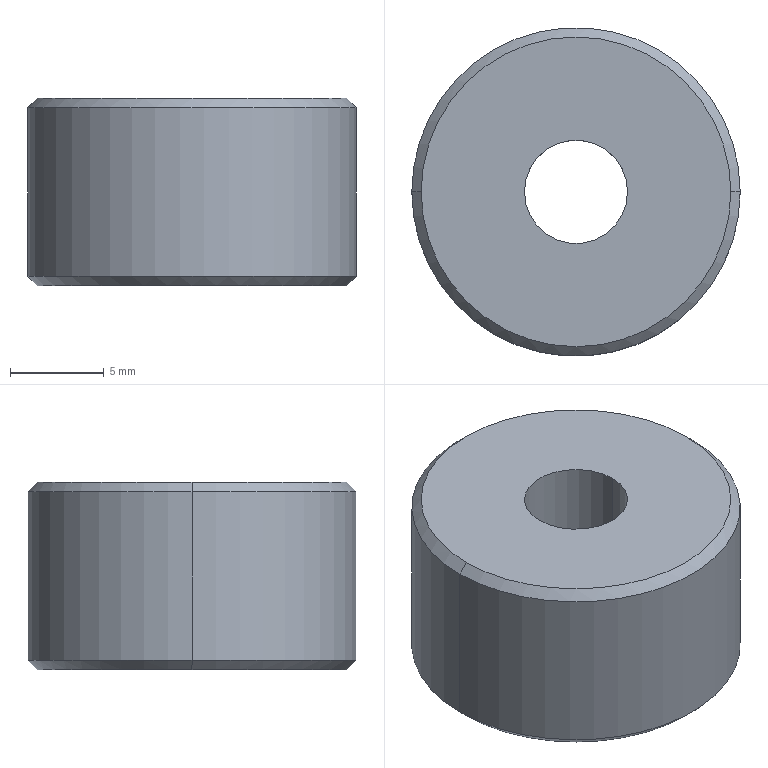Part | SolidWorks | features Chamfer 1, Extrusion 1, ICE 1 | 1 solid | 13 faces | box 17.5 x 17.5 x 10 mm | volume 1853 mm3 | cylinder 6 | cone 4 | plane 3 | commonest cylinder face diameters 5.5 x2 10 x2 17.5 x2
STEP:
#1=CARTESIAN_POINT('',(8.25,0.,10.));
#2=VERTEX_POINT('',#1);
#3=CARTESIAN_POINT('',(-8.25,0.,10.));
#4=VERTEX_POINT('',#3);
#5=CARTESIAN_POINT('',(0.,0.,10.));
#6=DIRECTION('',(0.,0.,1.));
#7=DIRECTION('',(1.,0.,0.));
#8=AXIS2_PLACEMENT_3D('',#5,#6,#7);
#9=CIRCLE('',#8,8.25);
#10=EDGE_CURVE('',#2,#4,#9,.T.);
#11=ORIENTED_EDGE('',*,*,#10,.F.);
#12=CARTESIAN_POINT('',(8.75,0.,9.5));
#13=VERTEX_POINT('',#12);
#14=CARTESIAN_POINT('',(8.25,0.,10.));
#15=DIRECTION('',(0.7071,0.,-0.7071));
#16=VECTOR('',#15,1000.);
#17=LINE('',#14,#16);
#18=EDGE_CURVE('',#2,#13,#17,.T.);
#19=ORIENTED_EDGE('',*,*,#18,.T.);
#20=CARTESIAN_POINT('',(-8.75,0.,9.5));
#21=VERTEX_POINT('',#20);
#22=CARTESIAN_POINT('',(0.,0.,9.5));
#23=DIRECTION('',(0.,0.,-1.));
#24=DIRECTION('',(1.,0.,0.));
#25=AXIS2_PLACEMENT_3D('',#22,#23,#24);
#26=CIRCLE('',#25,8.75);
#27=EDGE_CURVE('',#21,#13,#26,.T.);
#28=ORIENTED_EDGE('',*,*,#27,.F.);
#29=CARTESIAN_POINT('',(-8.25,0.,10.));
#30=DIRECTION('',(-0.7071,0.,-0.7071));
#31=VECTOR('',#30,1000.);
#32=LINE('',#29,#31);
#33=EDGE_CURVE('',#4,#21,#32,.T.);
#34=ORIENTED_EDGE('',*,*,#33,.F.);
#35=EDGE_LOOP('',(#11,#19,#28,#34));
#36=FACE_OUTER_BOUND('',#35,.T.);
#37=CARTESIAN_POINT('',(0.,0.,10.));
#38=DIRECTION('',(0.,0.,-1.));
#39=DIRECTION('',(-1.,0.,0.));
#40=AXIS2_PLACEMENT_3D('',#37,#38,#39);
#41=CONICAL_SURFACE('',#40,8.25,0.7854);
#42=ADVANCED_FACE('',(#36),#41,.T.);
#43=CARTESIAN_POINT('',(-8.25,0.,0.));
#44=VERTEX_POINT('',#43);
#45=CARTESIAN_POINT('',(8.25,0.,0.));
#46=VERTEX_POINT('',#45);
#47=CARTESIAN_POINT('',(0.,0.,0.));
#48=DIRECTION('',(0.,0.,-1.));
#49=DIRECTION('',(1.,0.,0.));
#50=AXIS2_PLACEMENT_3D('',#47,#48,#49);
#51=CIRCLE('',#50,8.25);
#52=EDGE_CURVE('',#44,#46,#51,.T.);
#53=ORIENTED_EDGE('',*,*,#52,.F.);
#54=CARTESIAN_POINT('',(-8.75,0.,0.5));
#55=VERTEX_POINT('',#54);
#56=CARTESIAN_POINT('',(-8.75,0.,0.5));
#57=DIRECTION('',(-0.7071,0.,0.7071));
#58=VECTOR('',#57,1000.);
#59=LINE('',#56,#58);
#60=EDGE_CURVE('',#44,#55,#59,.T.);
#61=ORIENTED_EDGE('',*,*,#60,.T.);
#62=CARTESIAN_POINT('',(8.75,0.,0.5));
#63=VERTEX_POINT('',#62);
#64=CARTESIAN_POINT('',(0.,0.,0.5));
#65=DIRECTION('',(0.,0.,1.));
#66=DIRECTION('',(1.,0.,0.));
#67=AXIS2_PLACEMENT_3D('',#64,#65,#66);
#68=CIRCLE('',#67,8.75);
#69=EDGE_CURVE('',#63,#55,#68,.T.);
#70=ORIENTED_EDGE('',*,*,#69,.F.);
#71=CARTESIAN_POINT('',(8.75,0.,0.5));
#72=DIRECTION('',(0.7071,0.,0.7071));
#73=VECTOR('',#72,1000.);
#74=LINE('',#71,#73);
#75=EDGE_CURVE('',#46,#63,#74,.T.);
#76=ORIENTED_EDGE('',*,*,#75,.F.);
#77=EDGE_LOOP('',(#53,#61,#70,#76));
#78=FACE_OUTER_BOUND('',#77,.T.);
#79=CARTESIAN_POINT('',(0.,0.,0.5));
#80=DIRECTION('',(0.,0.,1.));
#81=DIRECTION('',(1.,0.,0.));
#82=AXIS2_PLACEMENT_3D('',#79,#80,#81);
#83=CONICAL_SURFACE('',#82,8.75,0.7854);
#84=ADVANCED_FACE('',(#78),#83,.T.);
#85=CARTESIAN_POINT('',(5.,0.,5.5));
#86=VERTEX_POINT('',#85);
#87=CARTESIAN_POINT('',(-5.,0.,5.5));
#88=VERTEX_POINT('',#87);
#89=CARTESIAN_POINT('',(0.,0.,5.5));
#90=DIRECTION('',(0.,0.,-1.));
#91=DIRECTION('',(-1.,0.,0.));
#92=AXIS2_PLACEMENT_3D('',#89,#90,#91);
#93=CIRCLE('',#92,5.);
#94=EDGE_CURVE('',#86,#88,#93,.T.);
#95=ORIENTED_EDGE('',*,*,#94,.F.);
#96=CARTESIAN_POINT('',(5.,0.,0.));
#97=VERTEX_POINT('',#96);
#98=CARTESIAN_POINT('',(5.,0.,5.5));
#99=DIRECTION('',(0.,0.,-1.));
#100=VECTOR('',#99,1000.);
#101=LINE('',#98,#100);
#102=EDGE_CURVE('',#86,#97,#101,.T.);
#103=ORIENTED_EDGE('',*,*,#102,.T.);
#104=CARTESIAN_POINT('',(-5.,0.,0.));
#105=VERTEX_POINT('',#104);
#106=CARTESIAN_POINT('',(0.,0.,0.));
#107=DIRECTION('',(0.,0.,-1.));
#108=DIRECTION('',(-1.,0.,0.));
#109=AXIS2_PLACEMENT_3D('',#106,#107,#108);
#110=CIRCLE('',#109,5.);
#111=EDGE_CURVE('',#97,#105,#110,.T.);
#112=ORIENTED_EDGE('',*,*,#111,.T.);
#113=CARTESIAN_POINT('',(-5.,0.,5.5));
#114=DIRECTION('',(0.,0.,-1.));
#115=VECTOR('',#114,1000.);
#116=LINE('',#113,#115);
#117=EDGE_CURVE('',#88,#105,#116,.T.);
#118=ORIENTED_EDGE('',*,*,#117,.F.);
#119=EDGE_LOOP('',(#95,#103,#112,#118));
#120=FACE_OUTER_BOUND('',#119,.T.);
#121=CARTESIAN_POINT('',(0.,0.,5.5));
#122=DIRECTION('',(0.,0.,-1.));
#123=DIRECTION('',(-1.,0.,0.));
#124=AXIS2_PLACEMENT_3D('',#121,#122,#123);
#125=CYLINDRICAL_SURFACE('',#124,5.);
#126=ADVANCED_FACE('',(#120),#125,.F.);
#127=ORIENTED_EDGE('',*,*,#27,.T.);
#128=CARTESIAN_POINT('',(8.75,0.,10.));
#129=DIRECTION('',(0.,0.,-1.));
#130=VECTOR('',#129,1000.);
#131=LINE('',#128,#130);
#132=EDGE_CURVE('',#13,#63,#131,.T.);
#133=ORIENTED_EDGE('',*,*,#132,.T.);
#134=ORIENTED_EDGE('',*,*,#69,.T.);
#135=CARTESIAN_POINT('',(-8.75,0.,10.));
#136=DIRECTION('',(0.,0.,-1.));
#137=VECTOR('',#136,1000.);
#138=LINE('',#135,#137);
#139=EDGE_CURVE('',#21,#55,#138,.T.);
#140=ORIENTED_EDGE('',*,*,#139,.F.);
#141=EDGE_LOOP('',(#127,#133,#134,#140));
#142=FACE_OUTER_BOUND('',#141,.T.);
#143=CARTESIAN_POINT('',(0.,0.,10.));
#144=DIRECTION('',(0.,0.,-1.));
#145=DIRECTION('',(-1.,0.,0.));
#146=AXIS2_PLACEMENT_3D('',#143,#144,#145);
#147=CYLINDRICAL_SURFACE('',#146,8.75);
#148=ADVANCED_FACE('',(#142),#147,.T.);
#149=CARTESIAN_POINT('',(-2.75,0.,10.));
#150=VERTEX_POINT('',#149);
#151=CARTESIAN_POINT('',(2.75,0.,10.));
#152=VERTEX_POINT('',#151);
#153=CARTESIAN_POINT('',(0.,0.,10.));
#154=DIRECTION('',(0.,0.,1.));
#155=DIRECTION('',(1.,0.,0.));
#156=AXIS2_PLACEMENT_3D('',#153,#154,#155);
#157=CIRCLE('',#156,2.75);
#158=EDGE_CURVE('',#150,#152,#157,.T.);
#159=ORIENTED_EDGE('',*,*,#158,.T.);
#160=CARTESIAN_POINT('',(2.75,0.,5.5));
#161=VERTEX_POINT('',#160);
#162=CARTESIAN_POINT('',(2.75,0.,10.));
#163=DIRECTION('',(0.,0.,-1.));
#164=VECTOR('',#163,1000.);
#165=LINE('',#162,#164);
#166=EDGE_CURVE('',#152,#161,#165,.T.);
#167=ORIENTED_EDGE('',*,*,#166,.T.);
#168=CARTESIAN_POINT('',(-2.75,0.,5.5));
#169=VERTEX_POINT('',#168);
#170=CARTESIAN_POINT('',(0.,0.,5.5));
#171=DIRECTION('',(0.,0.,-1.));
#172=DIRECTION('',(-1.,0.,0.));
#173=AXIS2_PLACEMENT_3D('',#170,#171,#172);
#174=CIRCLE('',#173,2.75);
#175=EDGE_CURVE('',#161,#169,#174,.T.);
#176=ORIENTED_EDGE('',*,*,#175,.T.);
#177=CARTESIAN_POINT('',(-2.75,0.,10.));
#178=DIRECTION('',(0.,0.,-1.));
#179=VECTOR('',#178,1000.);
#180=LINE('',#177,#179);
#181=EDGE_CURVE('',#150,#169,#180,.T.);
#182=ORIENTED_EDGE('',*,*,#181,.F.);
#183=EDGE_LOOP('',(#159,#167,#176,#182));
#184=FACE_OUTER_BOUND('',#183,.T.);
#185=CARTESIAN_POINT('',(0.,0.,10.));
#186=DIRECTION('',(0.,0.,-1.));
#187=DIRECTION('',(-1.,0.,0.));
#188=AXIS2_PLACEMENT_3D('',#185,#186,#187);
#189=CYLINDRICAL_SURFACE('',#188,2.75);
#190=ADVANCED_FACE('',(#184),#189,.F.);
#191=ORIENTED_EDGE('',*,*,#166,.F.);
#192=CARTESIAN_POINT('',(0.,0.,10.));
#193=DIRECTION('',(0.,0.,1.));
#194=DIRECTION('',(1.,0.,0.));
#195=AXIS2_PLACEMENT_3D('',#192,#193,#194);
#196=CIRCLE('',#195,2.75);
#197=EDGE_CURVE('',#152,#150,#196,.T.);
#198=ORIENTED_EDGE('',*,*,#197,.T.);
#199=ORIENTED_EDGE('',*,*,#181,.T.);
#200=CARTESIAN_POINT('',(0.,0.,5.5));
#201=DIRECTION('',(0.,0.,-1.));
#202=DIRECTION('',(-1.,0.,0.));
#203=AXIS2_PLACEMENT_3D('',#200,#201,#202);
#204=CIRCLE('',#203,2.75);
#205=EDGE_CURVE('',#169,#161,#204,.T.);
#206=ORIENTED_EDGE('',*,*,#205,.T.);
#207=EDGE_LOOP('',(#191,#198,#199,#206));
#208=FACE_OUTER_BOUND('',#207,.T.);
#209=CARTESIAN_POINT('',(0.,0.,10.));
#210=DIRECTION('',(0.,0.,-1.));
#211=DIRECTION('',(-1.,0.,0.));
#212=AXIS2_PLACEMENT_3D('',#209,#210,#211);
#213=CYLINDRICAL_SURFACE('',#212,2.75);
#214=ADVANCED_FACE('',(#208),#213,.F.);
#215=CARTESIAN_POINT('',(0.,0.,10.));
#216=DIRECTION('',(0.,0.,1.));
#217=DIRECTION('',(1.,0.,0.));
#218=AXIS2_PLACEMENT_3D('',#215,#216,#217);
#219=CIRCLE('',#218,8.25);
#220=EDGE_CURVE('',#4,#2,#219,.T.);
#221=ORIENTED_EDGE('',*,*,#220,.T.);
#222=ORIENTED_EDGE('',*,*,#10,.T.);
#223=EDGE_LOOP('',(#221,#222));
#224=FACE_OUTER_BOUND('',#223,.T.);
#225=ORIENTED_EDGE('',*,*,#158,.F.);
#226=ORIENTED_EDGE('',*,*,#197,.F.);
#227=EDGE_LOOP('',(#225,#226));
#228=FACE_BOUND('',#227,.T.);
#229=CARTESIAN_POINT('',(0.,0.,10.));
#230=DIRECTION('',(0.,0.,1.));
#231=DIRECTION('',(1.,0.,0.));
#232=AXIS2_PLACEMENT_3D('',#229,#230,#231);
#233=PLANE('',#232);
#234=ADVANCED_FACE('',(#224,#228),#233,.T.);
#235=CARTESIAN_POINT('',(0.,0.,0.));
#236=DIRECTION('',(0.,0.,-1.));
#237=DIRECTION('',(1.,0.,0.));
#238=AXIS2_PLACEMENT_3D('',#235,#236,#237);
#239=CIRCLE('',#238,8.25);
#240=EDGE_CURVE('',#46,#44,#239,.T.);
#241=ORIENTED_EDGE('',*,*,#240,.T.);
#242=ORIENTED_EDGE('',*,*,#52,.T.);
#243=EDGE_LOOP('',(#241,#242));
#244=FACE_OUTER_BOUND('',#243,.T.);
#245=CARTESIAN_POINT('',(0.,0.,0.));
#246=DIRECTION('',(0.,0.,-1.));
#247=DIRECTION('',(-1.,0.,0.));
#248=AXIS2_PLACEMENT_3D('',#245,#246,#247);
#249=CIRCLE('',#248,5.);
#250=EDGE_CURVE('',#105,#97,#249,.T.);
#251=ORIENTED_EDGE('',*,*,#250,.F.);
#252=ORIENTED_EDGE('',*,*,#111,.F.);
#253=EDGE_LOOP('',(#251,#252));
#254=FACE_BOUND('',#253,.T.);
#255=CARTESIAN_POINT('',(0.,0.,0.));
#256=DIRECTION('',(0.,0.,1.));
#257=DIRECTION('',(1.,0.,0.));
#258=AXIS2_PLACEMENT_3D('',#255,#256,#257);
#259=PLANE('',#258);
#260=ADVANCED_FACE('',(#244,#254),#259,.F.);
#261=ORIENTED_EDGE('',*,*,#132,.F.);
#262=CARTESIAN_POINT('',(0.,0.,9.5));
#263=DIRECTION('',(0.,0.,-1.));
#264=DIRECTION('',(1.,0.,0.));
#265=AXIS2_PLACEMENT_3D('',#262,#263,#264);
#266=CIRCLE('',#265,8.75);
#267=EDGE_CURVE('',#13,#21,#266,.T.);
#268=ORIENTED_EDGE('',*,*,#267,.T.);
#269=ORIENTED_EDGE('',*,*,#139,.T.);
#270=CARTESIAN_POINT('',(0.,0.,0.5));
#271=DIRECTION('',(0.,0.,1.));
#272=DIRECTION('',(1.,0.,0.));
#273=AXIS2_PLACEMENT_3D('',#270,#271,#272);
#274=CIRCLE('',#273,8.75);
#275=EDGE_CURVE('',#55,#63,#274,.T.);
#276=ORIENTED_EDGE('',*,*,#275,.T.);
#277=EDGE_LOOP('',(#261,#268,#269,#276));
#278=FACE_OUTER_BOUND('',#277,.T.);
#279=CARTESIAN_POINT('',(0.,0.,10.));
#280=DIRECTION('',(0.,0.,-1.));
#281=DIRECTION('',(-1.,0.,0.));
#282=AXIS2_PLACEMENT_3D('',#279,#280,#281);
#283=CYLINDRICAL_SURFACE('',#282,8.75);
#284=ADVANCED_FACE('',(#278),#283,.T.);
#285=ORIENTED_EDGE('',*,*,#102,.F.);
#286=CARTESIAN_POINT('',(0.,0.,5.5));
#287=DIRECTION('',(0.,0.,-1.));
#288=DIRECTION('',(-1.,0.,0.));
#289=AXIS2_PLACEMENT_3D('',#286,#287,#288);
#290=CIRCLE('',#289,5.);
#291=EDGE_CURVE('',#88,#86,#290,.T.);
#292=ORIENTED_EDGE('',*,*,#291,.F.);
#293=ORIENTED_EDGE('',*,*,#117,.T.);
#294=ORIENTED_EDGE('',*,*,#250,.T.);
#295=EDGE_LOOP('',(#285,#292,#293,#294));
#296=FACE_OUTER_BOUND('',#295,.T.);
#297=CARTESIAN_POINT('',(0.,0.,5.5));
#298=DIRECTION('',(0.,0.,-1.));
#299=DIRECTION('',(-1.,0.,0.));
#300=AXIS2_PLACEMENT_3D('',#297,#298,#299);
#301=CYLINDRICAL_SURFACE('',#300,5.);
#302=ADVANCED_FACE('',(#296),#301,.F.);
#303=ORIENTED_EDGE('',*,*,#205,.F.);
#304=ORIENTED_EDGE('',*,*,#175,.F.);
#305=EDGE_LOOP('',(#303,#304));
#306=FACE_BOUND('',#305,.T.);
#307=ORIENTED_EDGE('',*,*,#291,.T.);
#308=ORIENTED_EDGE('',*,*,#94,.T.);
#309=EDGE_LOOP('',(#307,#308));
#310=FACE_OUTER_BOUND('',#309,.T.);
#311=CARTESIAN_POINT('',(0.,0.,5.5));
#312=DIRECTION('',(0.,0.,-1.));
#313=DIRECTION('',(-1.,0.,0.));
#314=AXIS2_PLACEMENT_3D('',#311,#312,#313);
#315=PLANE('',#314);
#316=ADVANCED_FACE('',(#306,#310),#315,.T.);
#317=ORIENTED_EDGE('',*,*,#60,.F.);
#318=ORIENTED_EDGE('',*,*,#240,.F.);
#319=ORIENTED_EDGE('',*,*,#75,.T.);
#320=ORIENTED_EDGE('',*,*,#275,.F.);
#321=EDGE_LOOP('',(#317,#318,#319,#320));
#322=FACE_OUTER_BOUND('',#321,.T.);
#323=CARTESIAN_POINT('',(0.,0.,0.5));
#324=DIRECTION('',(0.,0.,1.));
#325=DIRECTION('',(1.,0.,0.));
#326=AXIS2_PLACEMENT_3D('',#323,#324,#325);
#327=CONICAL_SURFACE('',#326,8.75,0.7854);
#328=ADVANCED_FACE('',(#322),#327,.T.);
#329=ORIENTED_EDGE('',*,*,#18,.F.);
#330=ORIENTED_EDGE('',*,*,#220,.F.);
#331=ORIENTED_EDGE('',*,*,#33,.T.);
#332=ORIENTED_EDGE('',*,*,#267,.F.);
#333=EDGE_LOOP('',(#329,#330,#331,#332));
#334=FACE_OUTER_BOUND('',#333,.T.);
#335=CARTESIAN_POINT('',(0.,0.,10.));
#336=DIRECTION('',(0.,0.,-1.));
#337=DIRECTION('',(-1.,0.,0.));
#338=AXIS2_PLACEMENT_3D('',#335,#336,#337);
#339=CONICAL_SURFACE('',#338,8.25,0.7854);
#340=ADVANCED_FACE('',(#334),#339,.T.);
#341=CLOSED_SHELL('',(#42,#84,#126,#148,#190,#214,#234,#260,#284,#302,#316,#328,#340));
#342=MANIFOLD_SOLID_BREP('',#341);
#343=CARTESIAN_POINT('',(0.,0.,0.));
#344=DIRECTION('',(0.,0.,1.));
#345=DIRECTION('',(1.,0.,0.));
#346=AXIS2_PLACEMENT_3D('',#343,#344,#345);
#347=(LENGTH_UNIT()NAMED_UNIT(*)SI_UNIT(.MILLI.,.METRE.));
#348=UNCERTAINTY_MEASURE_WITH_UNIT(LENGTH_MEASURE(0.00001),#347,'','');
#349=(NAMED_UNIT(*)PLANE_ANGLE_UNIT()SI_UNIT($,.RADIAN.));
#350=(NAMED_UNIT(*)SI_UNIT($,.STERADIAN.)SOLID_ANGLE_UNIT());
#351=(GEOMETRIC_REPRESENTATION_CONTEXT(3)GLOBAL_UNCERTAINTY_ASSIGNED_CONTEXT((#348))GLOBAL_UNIT_ASSIGNED_CONTEXT((#347,#349,#350))REPRESENTATION_CONTEXT('',''));
#352=ADVANCED_BREP_SHAPE_REPRESENTATION('',(#342,#346),#351);